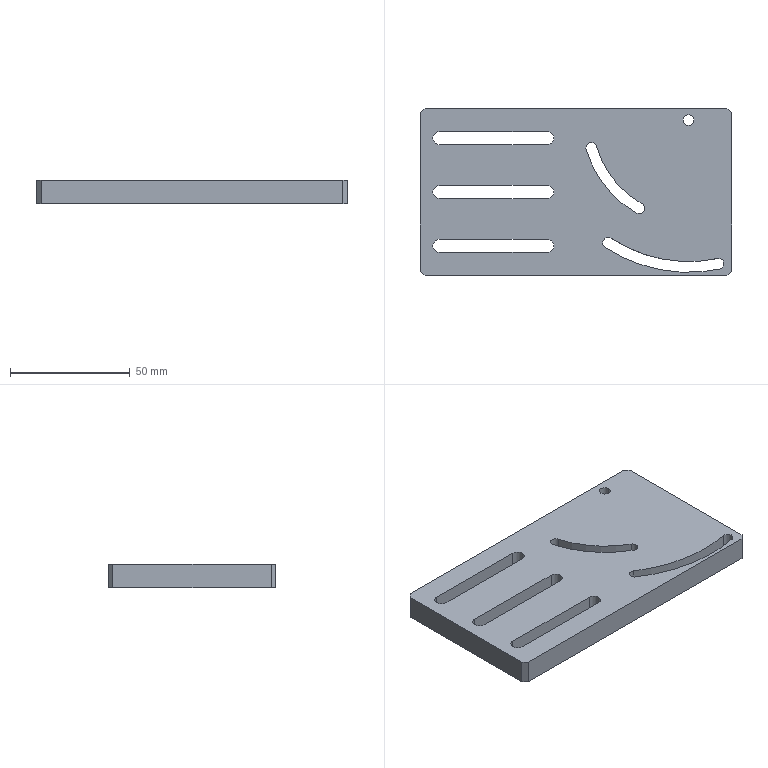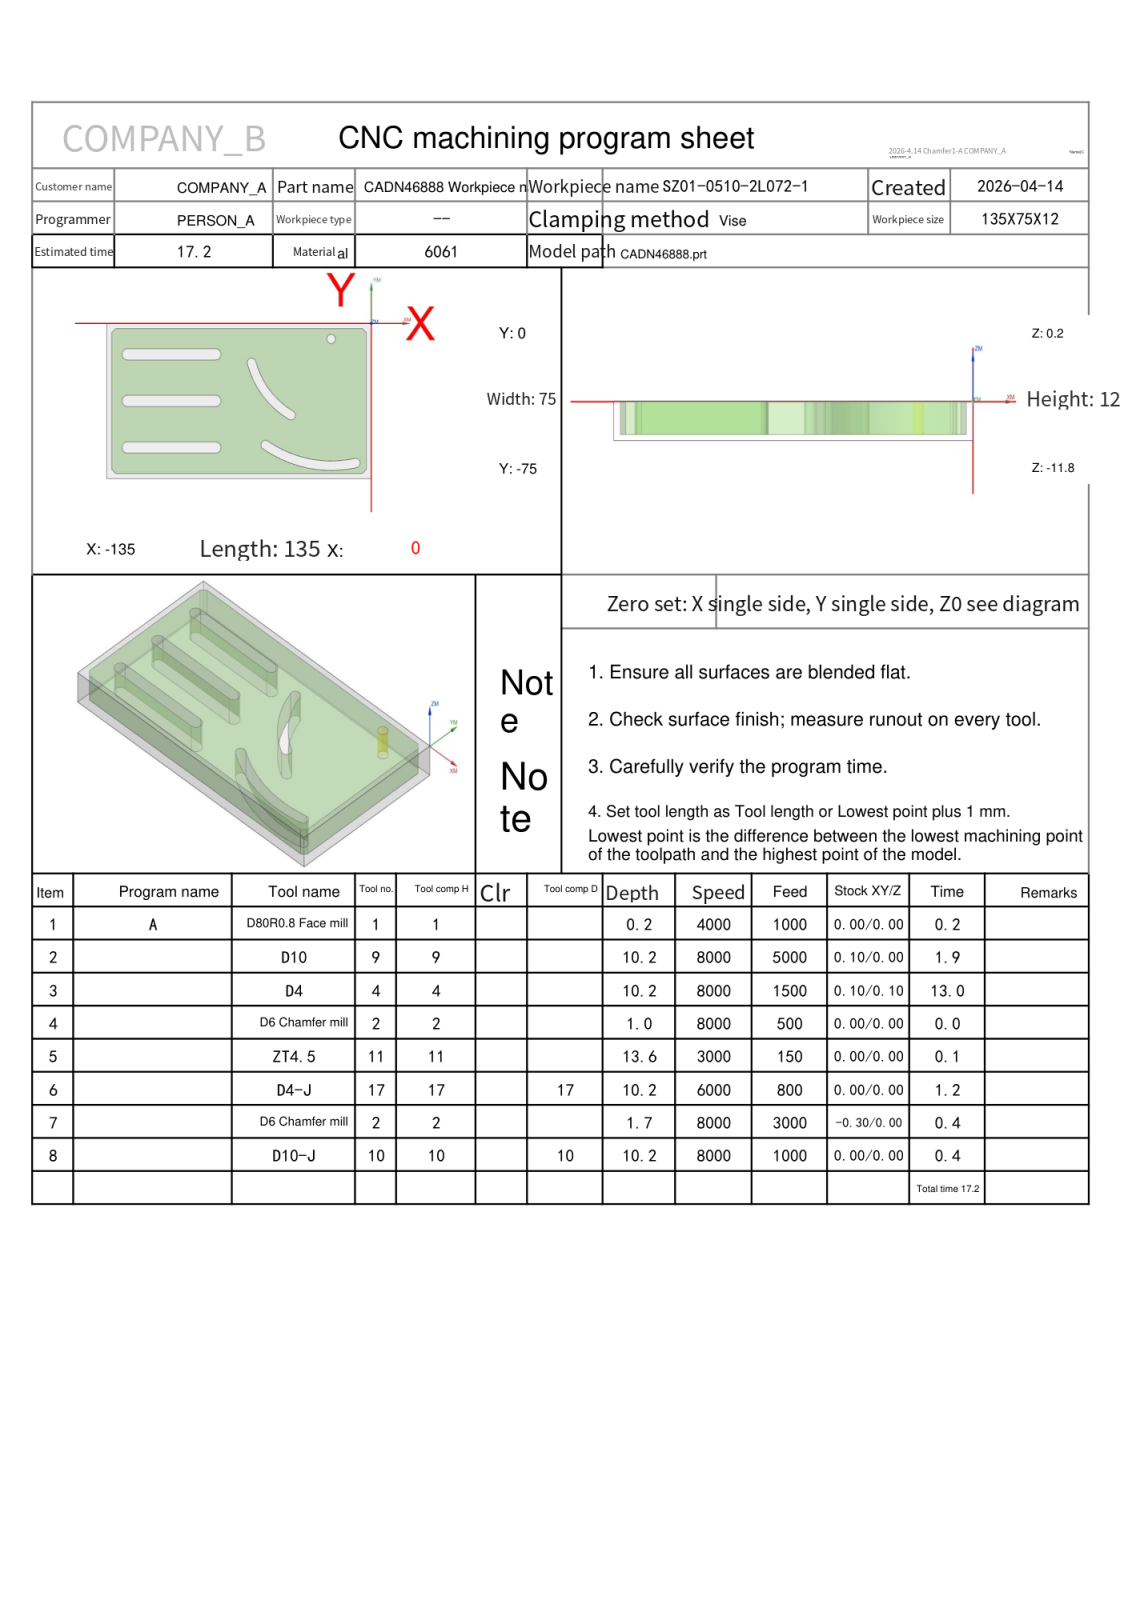NC program | NX | posted by the shop | part box 130 x 70 x 10 mm
Lines 448 to 1256 of 2533:
N5 T04 M06
(D4  D=4. R=0. H=04 ce=0.10 di=0.10)
G00 G90 G54 X-102. Y-60.65 M03 S8000
G43 H04 Z20.
M08
Z.5
G01 X-79.5 Z.442 F2500.
G03 X-78.85 Y-60. Z.439 I0.0 J.65
X-79.5 Y-59.35 Z.436 I-.65 J0.0
G01 X-124.5 Z.32
G03 X-125.15 Y-60. Z.317 I0.0 J-.65
X-124.89 Y-60.52 Z.315 I.65 J0.0
X-124.5 Y-60.65 Z.314 I.39 J.52
G01 X-79.5 Z.197
G03 X-78.85 Y-60. Z.195 I0.0 J.65
X-79.5 Y-59.35 Z.192 I-.65 J0.0
G01 X-124.5 Z.075
G03 X-125.15 Y-60. Z.073 I0.0 J-.65
X-124.89 Y-60.52 Z.071 I.65 J0.0
X-124.5 Y-60.65 Z.07 I.39 J.52
G01 X-79.5 Z-.047
G03 X-78.85 Y-60. Z-.049 I0.0 J.65
X-79.5 Y-59.35 Z-.052 I-.65 J0.0
G01 X-124.5 Z-.169
G03 X-125.15 Y-60. Z-.172 I0.0 J-.65
X-124.89 Y-60.52 Z-.173 I.65 J0.0
X-124.5 Y-60.65 Z-.174 I.39 J.52
G01 X-79.5 Z-.291
G03 X-78.85 Y-60. Z-.294 I0.0 J.65
X-79.5 Y-59.35 Z-.296 I-.65 J0.0
G01 X-124.5 Z-.413
G03 X-125.15 Y-60. Z-.416 I0.0 J-.65
X-124.89 Y-60.52 Z-.417 I.65 J0.0
X-124.5 Y-60.65 Z-.418 I.39 J.52
G01 X-79.5 Z-.535
G03 X-78.85 Y-60. Z-.538 I0.0 J.65
X-79.5 Y-59.35 Z-.54 I-.65 J0.0
G01 X-124.5 Z-.657
G03 X-125.15 Y-60. Z-.66 I0.0 J-.65
X-124.89 Y-60.52 Z-.661 I.65 J0.0
X-124.5 Y-60.65 Z-.663 I.39 J.52
G01 X-79.5 Z-.779
G03 X-78.85 Y-60. Z-.782 I0.0 J.65
X-79.5 Y-59.35 Z-.785 I-.65 J0.0
G01 X-124.5 Z-.901
G03 X-125.15 Y-60. Z-.904 I0.0 J-.65
X-124.89 Y-60.52 Z-.906 I.65 J0.0
X-124.5 Y-60.65 Z-.907 I.39 J.52
G01 X-79.5 Z-1.024
G03 X-78.85 Y-60. Z-1.026 I0.0 J.65
X-79.5 Y-59.35 Z-1.029 I-.65 J0.0
G01 X-124.5 Z-1.146
G03 X-125.15 Y-60. Z-1.148 I0.0 J-.65
X-124.89 Y-60.52 Z-1.15 I.65 J0.0
X-124.5 Y-60.65 Z-1.151 I.39 J.52
G01 X-79.5 Z-1.268
G03 X-78.85 Y-60. Z-1.27 I0.0 J.65
X-79.5 Y-59.35 Z-1.273 I-.65 J0.0
G01 X-124.5 Z-1.39
G03 X-125.15 Y-60. Z-1.392 I0.0 J-.65
X-124.89 Y-60.52 Z-1.394 I.65 J0.0
X-124.5 Y-60.65 Z-1.395 I.39 J.52
G01 X-79.5 Z-1.512
G03 X-78.85 Y-60. Z-1.515 I0.0 J.65
X-79.5 Y-59.35 Z-1.517 I-.65 J0.0
G01 X-124.5 Z-1.634
G03 X-125.15 Y-60. Z-1.637 I0.0 J-.65
X-124.89 Y-60.52 Z-1.638 I.65 J0.0
X-124.5 Y-60.65 Z-1.639 I.39 J.52
G01 X-79.5 Z-1.756
G03 X-78.85 Y-60. Z-1.759 I0.0 J.65
X-79.5 Y-59.35 Z-1.761 I-.65 J0.0
G01 X-124.5 Z-1.878
G03 X-125.15 Y-60. Z-1.881 I0.0 J-.65
X-124.89 Y-60.52 Z-1.882 I.65 J0.0
X-124.5 Y-60.65 Z-1.883 I.39 J.52
G01 X-79.5 Z-2.
G03 X-78.85 Y-60. Z-2.003 I0.0 J.65
X-79.5 Y-59.35 Z-2.006 I-.65 J0.0
G01 X-124.5 Z-2.122
G03 X-125.15 Y-60. Z-2.125 I0.0 J-.65
X-124.89 Y-60.52 Z-2.127 I.65 J0.0
X-124.5 Y-60.65 Z-2.128 I.39 J.52
G01 X-79.5 Z-2.244
G03 X-78.85 Y-60. Z-2.247 I0.0 J.65
X-79.5 Y-59.35 Z-2.25 I-.65 J0.0
G01 X-124.5 Z-2.367
G03 X-125.15 Y-60. Z-2.369 I0.0 J-.65
X-124.89 Y-60.52 Z-2.371 I.65 J0.0
X-124.5 Y-60.65 Z-2.372 I.39 J.52
G01 X-79.5 Z-2.489
G03 X-78.85 Y-60. Z-2.491 I0.0 J.65
X-79.5 Y-59.35 Z-2.494 I-.65 J0.0
G01 X-124.5 Z-2.611
G03 X-125.15 Y-60. Z-2.613 I0.0 J-.65
X-124.89 Y-60.52 Z-2.615 I.65 J0.0
X-124.5 Y-60.65 Z-2.616 I.39 J.52
G01 X-79.5 Z-2.733
G03 X-78.85 Y-60. Z-2.735 I0.0 J.65
X-79.5 Y-59.35 Z-2.738 I-.65 J0.0
G01 X-124.5 Z-2.855
G03 X-125.15 Y-60. Z-2.858 I0.0 J-.65
X-124.89 Y-60.52 Z-2.859 I.65 J0.0
X-124.5 Y-60.65 Z-2.86 I.39 J.52
G01 X-79.5 Z-2.977
G03 X-78.85 Y-60. Z-2.98 I0.0 J.65
X-79.5 Y-59.35 Z-2.982 I-.65 J0.0
G01 X-124.5 Z-3.099
G03 X-125.15 Y-60. Z-3.102 I0.0 J-.65
X-124.89 Y-60.52 Z-3.103 I.65 J0.0
X-124.5 Y-60.65 Z-3.104 I.39 J.52
G01 X-79.5 Z-3.221
G03 X-78.85 Y-60. Z-3.224 I0.0 J.65
X-79.5 Y-59.35 Z-3.226 I-.65 J0.0
G01 X-124.5 Z-3.343
G03 X-125.15 Y-60. Z-3.346 I0.0 J-.65
X-124.89 Y-60.52 Z-3.347 I.65 J0.0
X-124.5 Y-60.65 Z-3.349 I.39 J.52
G01 X-79.5 Z-3.465
G03 X-78.85 Y-60. Z-3.468 I0.0 J.65
X-79.5 Y-59.35 Z-3.471 I-.65 J0.0
G01 X-124.5 Z-3.587
G03 X-125.15 Y-60. Z-3.59 I0.0 J-.65
X-124.89 Y-60.52 Z-3.592 I.65 J0.0
X-124.5 Y-60.65 Z-3.593 I.39 J.52
G01 X-79.5 Z-3.71
G03 X-78.85 Y-60. Z-3.712 I0.0 J.65
X-79.5 Y-59.35 Z-3.715 I-.65 J0.0
G01 X-124.5 Z-3.832
G03 X-125.15 Y-60. Z-3.834 I0.0 J-.65
X-124.89 Y-60.52 Z-3.836 I.65 J0.0
X-124.5 Y-60.65 Z-3.837 I.39 J.52
G01 X-79.5 Z-3.954
G03 X-78.85 Y-60. Z-3.956 I0.0 J.65
X-79.5 Y-59.35 Z-3.959 I-.65 J0.0
G01 X-124.5 Z-4.076
G03 X-125.15 Y-60. Z-4.078 I0.0 J-.65
X-124.89 Y-60.52 Z-4.08 I.65 J0.0
X-124.5 Y-60.65 Z-4.081 I.39 J.52
G01 X-79.5 Z-4.198
G03 X-78.85 Y-60. Z-4.201 I0.0 J.65
X-79.5 Y-59.35 Z-4.203 I-.65 J0.0
G01 X-124.5 Z-4.32
G03 X-125.15 Y-60. Z-4.323 I0.0 J-.65
X-124.89 Y-60.52 Z-4.324 I.65 J0.0
X-124.5 Y-60.65 Z-4.325 I.39 J.52
G01 X-79.5 Z-4.442
G03 X-78.85 Y-60. Z-4.445 I0.0 J.65
X-79.5 Y-59.35 Z-4.447 I-.65 J0.0
G01 X-124.5 Z-4.564
G03 X-125.15 Y-60. Z-4.567 I0.0 J-.65
X-124.89 Y-60.52 Z-4.568 I.65 J0.0
X-124.5 Y-60.65 Z-4.57 I.39 J.52
G01 X-79.5 Z-4.686
G03 X-78.85 Y-60. Z-4.689 I0.0 J.65
X-79.5 Y-59.35 Z-4.692 I-.65 J0.0
G01 X-124.5 Z-4.808
G03 X-125.15 Y-60. Z-4.811 I0.0 J-.65
X-124.89 Y-60.52 Z-4.813 I.65 J0.0
X-124.5 Y-60.65 Z-4.814 I.39 J.52
G01 X-79.5 Z-4.93
G03 X-78.85 Y-60. Z-4.933 I0.0 J.65
X-79.5 Y-59.35 Z-4.936 I-.65 J0.0
G01 X-124.5 Z-5.053
G03 X-125.15 Y-60. Z-5.055 I0.0 J-.65
X-124.89 Y-60.52 Z-5.057 I.65 J0.0
X-124.5 Y-60.65 Z-5.058 I.39 J.52
G01 X-79.5 Z-5.175
G03 X-78.85 Y-60. Z-5.177 I0.0 J.65
X-79.5 Y-59.35 Z-5.18 I-.65 J0.0
G01 X-124.5 Z-5.297
G03 X-125.15 Y-60. Z-5.299 I0.0 J-.65
X-124.89 Y-60.52 Z-5.301 I.65 J0.0
X-124.5 Y-60.65 Z-5.302 I.39 J.52
G01 X-79.5 Z-5.419
G03 X-78.85 Y-60. Z-5.422 I0.0 J.65
X-79.5 Y-59.35 Z-5.424 I-.65 J0.0
G01 X-124.5 Z-5.541
G03 X-125.15 Y-60. Z-5.544 I0.0 J-.65
X-124.89 Y-60.52 Z-5.545 I.65 J0.0
X-124.5 Y-60.65 Z-5.546 I.39 J.52
G01 X-79.5 Z-5.663
G03 X-78.85 Y-60. Z-5.666 I0.0 J.65
X-79.5 Y-59.35 Z-5.668 I-.65 J0.0
G01 X-124.5 Z-5.785
G03 X-125.15 Y-60. Z-5.788 I0.0 J-.65
X-124.89 Y-60.52 Z-5.789 I.65 J0.0
X-124.5 Y-60.65 Z-5.79 I.39 J.52
G01 X-79.5 Z-5.907
G03 X-78.85 Y-60. Z-5.91 I0.0 J.65
X-79.5 Y-59.35 Z-5.913 I-.65 J0.0
G01 X-124.5 Z-6.029
G03 X-125.15 Y-60. Z-6.032 I0.0 J-.65
X-124.89 Y-60.52 Z-6.034 I.65 J0.0
X-124.5 Y-60.65 Z-6.035 I.39 J.52
G01 X-79.5 Z-6.151
G03 X-78.85 Y-60. Z-6.154 I0.0 J.65
X-79.5 Y-59.35 Z-6.157 I-.65 J0.0
G01 X-124.5 Z-6.274
G03 X-125.15 Y-60. Z-6.276 I0.0 J-.65
X-124.89 Y-60.52 Z-6.278 I.65 J0.0
X-124.5 Y-60.65 Z-6.279 I.39 J.52
G01 X-79.5 Z-6.396
G03 X-78.85 Y-60. Z-6.398 I0.0 J.65
X-79.5 Y-59.35 Z-6.401 I-.65 J0.0
G01 X-124.5 Z-6.518
G03 X-125.15 Y-60. Z-6.52 I0.0 J-.65
X-124.89 Y-60.52 Z-6.522 I.65 J0.0
X-124.5 Y-60.65 Z-6.523 I.39 J.52
G01 X-79.5 Z-6.64
G03 X-78.85 Y-60. Z-6.642 I0.0 J.65
X-79.5 Y-59.35 Z-6.645 I-.65 J0.0
G01 X-124.5 Z-6.762
G03 X-125.15 Y-60. Z-6.765 I0.0 J-.65
X-124.89 Y-60.52 Z-6.766 I.65 J0.0
X-124.5 Y-60.65 Z-6.767 I.39 J.52
G01 X-79.5 Z-6.884
G03 X-78.85 Y-60. Z-6.887 I0.0 J.65
X-79.5 Y-59.35 Z-6.889 I-.65 J0.0
G01 X-124.5 Z-7.006
G03 X-125.15 Y-60. Z-7.009 I0.0 J-.65
X-124.89 Y-60.52 Z-7.01 I.65 J0.0
X-124.5 Y-60.65 Z-7.011 I.39 J.52
G01 X-79.5 Z-7.128
G03 X-78.85 Y-60. Z-7.131 I0.0 J.65
X-79.5 Y-59.35 Z-7.133 I-.65 J0.0
G01 X-124.5 Z-7.25
G03 X-125.15 Y-60. Z-7.253 I0.0 J-.65
X-124.89 Y-60.52 Z-7.254 I.65 J0.0
X-124.5 Y-60.65 Z-7.256 I.39 J.52
G01 X-79.5 Z-7.372
G03 X-78.85 Y-60. Z-7.375 I0.0 J.65
X-79.5 Y-59.35 Z-7.378 I-.65 J0.0
G01 X-124.5 Z-7.494
G03 X-125.15 Y-60. Z-7.497 I0.0 J-.65
X-124.89 Y-60.52 Z-7.499 I.65 J0.0
X-124.5 Y-60.65 Z-7.5 I.39 J.52
G01 X-79.5 Z-7.617
G03 X-78.85 Y-60. Z-7.619 I0.0 J.65
X-79.5 Y-59.35 Z-7.622 I-.65 J0.0
G01 X-124.5 Z-7.739
G03 X-125.15 Y-60. Z-7.741 I0.0 J-.65
X-124.89 Y-60.52 Z-7.743 I.65 J0.0
X-124.5 Y-60.65 Z-7.744 I.39 J.52
G01 X-79.5 Z-7.861
G03 X-78.85 Y-60. Z-7.863 I0.0 J.65
X-79.5 Y-59.35 Z-7.866 I-.65 J0.0
G01 X-124.5 Z-7.983
G03 X-125.15 Y-60. Z-7.985 I0.0 J-.65
X-124.89 Y-60.52 Z-7.987 I.65 J0.0
X-124.5 Y-60.65 Z-7.988 I.39 J.52
G01 X-79.5 Z-8.105
G03 X-78.85 Y-60. Z-8.108 I0.0 J.65
X-79.5 Y-59.35 Z-8.11 I-.65 J0.0
G01 X-124.5 Z-8.227
G03 X-125.15 Y-60. Z-8.23 I0.0 J-.65
X-124.89 Y-60.52 Z-8.231 I.65 J0.0
X-124.5 Y-60.65 Z-8.232 I.39 J.52
G01 X-79.5 Z-8.349
G03 X-78.85 Y-60. Z-8.352 I0.0 J.65
X-79.5 Y-59.35 Z-8.354 I-.65 J0.0
G01 X-124.5 Z-8.471
G03 X-125.15 Y-60. Z-8.474 I0.0 J-.65
X-124.89 Y-60.52 Z-8.475 I.65 J0.0
X-124.5 Y-60.65 Z-8.476 I.39 J.52
G01 X-79.5 Z-8.593
G03 X-78.85 Y-60. Z-8.596 I0.0 J.65
X-79.5 Y-59.35 Z-8.599 I-.65 J0.0
G01 X-124.5 Z-8.715
G03 X-125.15 Y-60. Z-8.718 I0.0 J-.65
X-124.89 Y-60.52 Z-8.72 I.65 J0.0
X-124.5 Y-60.65 Z-8.721 I.39 J.52
G01 X-79.5 Z-8.837
G03 X-78.85 Y-60. Z-8.84 I0.0 J.65
X-79.5 Y-59.35 Z-8.843 I-.65 J0.0
G01 X-124.5 Z-8.96
G03 X-125.15 Y-60. Z-8.962 I0.0 J-.65
X-124.89 Y-60.52 Z-8.964 I.65 J0.0
X-124.5 Y-60.65 Z-8.965 I.39 J.52
G01 X-79.5 Z-9.082
G03 X-78.85 Y-60. Z-9.084 I0.0 J.65
X-79.5 Y-59.35 Z-9.087 I-.65 J0.0
G01 X-124.5 Z-9.204
G03 X-125.15 Y-60. Z-9.206 I0.0 J-.65
X-124.89 Y-60.52 Z-9.208 I.65 J0.0
X-124.5 Y-60.65 Z-9.209 I.39 J.52
G01 X-79.5 Z-9.326
G03 X-78.85 Y-60. Z-9.328 I0.0 J.65
X-79.5 Y-59.35 Z-9.331 I-.65 J0.0
G01 X-124.5 Z-9.448
G03 X-125.15 Y-60. Z-9.451 I0.0 J-.65
X-124.89 Y-60.52 Z-9.452 I.65 J0.0
X-124.5 Y-60.65 Z-9.453 I.39 J.52
G01 X-79.5 Z-9.57
G03 X-78.85 Y-60. Z-9.573 I0.0 J.65
X-79.5 Y-59.35 Z-9.575 I-.65 J0.0
G01 X-124.5 Z-9.692
G03 X-125.15 Y-60. Z-9.695 I0.0 J-.65
X-124.89 Y-60.52 Z-9.696 I.65 J0.0
X-124.5 Y-60.65 Z-9.697 I.39 J.52
G01 X-79.5 Z-9.814
G03 X-78.85 Y-60. Z-9.817 I0.0 J.65
X-79.5 Y-59.35 Z-9.82 I-.65 J0.0
G01 X-124.5 Z-9.936
G03 X-125.15 Y-60. Z-9.939 I0.0 J-.65
X-124.89 Y-60.52 Z-9.941 I.65 J0.0
X-124.5 Y-60.65 Z-9.942 I.39 J.52
G01 X-102. Z-10.
X-79.5
G03 X-78.85 Y-60. I0.0 J.65
X-79.5 Y-59.35 I-.65 J0.0
G01 X-124.5
G03 X-125.15 Y-60. I0.0 J-.65
X-124.5 Y-60.65 I.65 J0.0
G01 X-102.
X-101.5
Z-9.
G00 Z20.
X-102. Y-36.85
Z.5
G01 X-124.5 Z.442
G03 X-125.15 Y-37.5 Z.439 I0.0 J-.65
X-124.5 Y-38.15 Z.436 I.65 J0.0
G01 X-79.5 Z.32
G03 X-78.85 Y-37.5 Z.317 I0.0 J.65
X-79.5 Y-36.85 Z.314 I-.65 J0.0
G01 X-124.5 Z.197
G03 X-125.15 Y-37.5 Z.195 I0.0 J-.65
X-124.5 Y-38.15 Z.192 I.65 J0.0
G01 X-79.5 Z.075
G03 X-78.85 Y-37.5 Z.073 I0.0 J.65
X-79.5 Y-36.85 Z.07 I-.65 J0.0
G01 X-124.5 Z-.047
G03 X-125.15 Y-37.5 Z-.049 I0.0 J-.65
X-124.5 Y-38.15 Z-.052 I.65 J0.0
G01 X-79.5 Z-.169
G03 X-78.85 Y-37.5 Z-.172 I0.0 J.65
X-79.5 Y-36.85 Z-.174 I-.65 J0.0
G01 X-124.5 Z-.291
G03 X-125.15 Y-37.5 Z-.294 I0.0 J-.65
X-124.5 Y-38.15 Z-.296 I.65 J0.0
G01 X-79.5 Z-.413
G03 X-78.85 Y-37.5 Z-.416 I0.0 J.65
X-79.5 Y-36.85 Z-.418 I-.65 J0.0
G01 X-124.5 Z-.535
G03 X-125.15 Y-37.5 Z-.538 I0.0 J-.65
X-124.5 Y-38.15 Z-.54 I.65 J0.0
G01 X-79.5 Z-.657
G03 X-78.85 Y-37.5 Z-.66 I0.0 J.65
X-79.5 Y-36.85 Z-.663 I-.65 J0.0
G01 X-124.5 Z-.779
G03 X-125.15 Y-37.5 Z-.782 I0.0 J-.65
X-124.5 Y-38.15 Z-.785 I.65 J0.0
G01 X-79.5 Z-.901
G03 X-78.85 Y-37.5 Z-.904 I0.0 J.65
X-79.5 Y-36.85 Z-.907 I-.65 J0.0
G01 X-124.5 Z-1.024
G03 X-125.15 Y-37.5 Z-1.026 I0.0 J-.65
X-124.5 Y-38.15 Z-1.029 I.65 J0.0
G01 X-79.5 Z-1.146
G03 X-78.85 Y-37.5 Z-1.148 I0.0 J.65
X-79.5 Y-36.85 Z-1.151 I-.65 J0.0
G01 X-124.5 Z-1.268
G03 X-125.15 Y-37.5 Z-1.27 I0.0 J-.65
X-124.5 Y-38.15 Z-1.273 I.65 J0.0
G01 X-79.5 Z-1.39
G03 X-78.85 Y-37.5 Z-1.392 I0.0 J.65
X-79.5 Y-36.85 Z-1.395 I-.65 J0.0
G01 X-124.5 Z-1.512
G03 X-125.15 Y-37.5 Z-1.515 I0.0 J-.65
X-124.5 Y-38.15 Z-1.517 I.65 J0.0
G01 X-79.5 Z-1.634
G03 X-78.85 Y-37.5 Z-1.637 I0.0 J.65
X-79.5 Y-36.85 Z-1.639 I-.65 J0.0
G01 X-124.5 Z-1.756
G03 X-125.15 Y-37.5 Z-1.759 I0.0 J-.65
X-124.5 Y-38.15 Z-1.761 I.65 J0.0
G01 X-79.5 Z-1.878
G03 X-78.85 Y-37.5 Z-1.881 I0.0 J.65
X-79.5 Y-36.85 Z-1.883 I-.65 J0.0
G01 X-124.5 Z-2.
G03 X-125.15 Y-37.5 Z-2.003 I0.0 J-.65
X-124.5 Y-38.15 Z-2.006 I.65 J0.0
G01 X-79.5 Z-2.122
G03 X-78.85 Y-37.5 Z-2.125 I0.0 J.65
X-79.5 Y-36.85 Z-2.128 I-.65 J0.0
G01 X-124.5 Z-2.244
G03 X-125.15 Y-37.5 Z-2.247 I0.0 J-.65
X-124.5 Y-38.15 Z-2.25 I.65 J0.0
G01 X-79.5 Z-2.367
G03 X-78.85 Y-37.5 Z-2.369 I0.0 J.65
X-79.5 Y-36.85 Z-2.372 I-.65 J0.0
G01 X-124.5 Z-2.489
G03 X-125.15 Y-37.5 Z-2.491 I0.0 J-.65
X-124.5 Y-38.15 Z-2.494 I.65 J0.0
G01 X-79.5 Z-2.611
G03 X-78.85 Y-37.5 Z-2.613 I0.0 J.65
X-79.5 Y-36.85 Z-2.616 I-.65 J0.0
G01 X-124.5 Z-2.733
G03 X-125.15 Y-37.5 Z-2.735 I0.0 J-.65
X-124.5 Y-38.15 Z-2.738 I.65 J0.0
G01 X-79.5 Z-2.855
G03 X-78.85 Y-37.5 Z-2.858 I0.0 J.65
X-79.5 Y-36.85 Z-2.86 I-.65 J0.0
G01 X-124.5 Z-2.977
G03 X-125.15 Y-37.5 Z-2.98 I0.0 J-.65
X-124.5 Y-38.15 Z-2.982 I.65 J0.0
G01 X-79.5 Z-3.099
G03 X-78.85 Y-37.5 Z-3.102 I0.0 J.65
X-79.5 Y-36.85 Z-3.104 I-.65 J0.0
G01 X-124.5 Z-3.221
G03 X-125.15 Y-37.5 Z-3.224 I0.0 J-.65
X-124.5 Y-38.15 Z-3.226 I.65 J0.0
G01 X-79.5 Z-3.343
G03 X-78.85 Y-37.5 Z-3.346 I0.0 J.65
X-79.5 Y-36.85 Z-3.349 I-.65 J0.0
G01 X-124.5 Z-3.465
G03 X-125.15 Y-37.5 Z-3.468 I0.0 J-.65
X-124.5 Y-38.15 Z-3.471 I.65 J0.0
G01 X-79.5 Z-3.587
G03 X-78.85 Y-37.5 Z-3.59 I0.0 J.65
X-79.5 Y-36.85 Z-3.593 I-.65 J0.0
G01 X-124.5 Z-3.71
G03 X-125.15 Y-37.5 Z-3.712 I0.0 J-.65
X-124.5 Y-38.15 Z-3.715 I.65 J0.0
G01 X-79.5 Z-3.832
G03 X-78.85 Y-37.5 Z-3.834 I0.0 J.65
X-79.5 Y-36.85 Z-3.837 I-.65 J0.0
G01 X-124.5 Z-3.954
G03 X-125.15 Y-37.5 Z-3.956 I0.0 J-.65
X-124.5 Y-38.15 Z-3.959 I.65 J0.0
G01 X-79.5 Z-4.076
G03 X-78.85 Y-37.5 Z-4.078 I0.0 J.65
X-79.5 Y-36.85 Z-4.081 I-.65 J0.0
G01 X-124.5 Z-4.198
G03 X-125.15 Y-37.5 Z-4.201 I0.0 J-.65
X-124.5 Y-38.15 Z-4.203 I.65 J0.0
G01 X-79.5 Z-4.32
G03 X-78.85 Y-37.5 Z-4.323 I0.0 J.65
X-79.5 Y-36.85 Z-4.325 I-.65 J0.0
G01 X-124.5 Z-4.442
G03 X-125.15 Y-37.5 Z-4.445 I0.0 J-.65
X-124.5 Y-38.15 Z-4.447 I.65 J0.0
G01 X-79.5 Z-4.564
G03 X-78.85 Y-37.5 Z-4.567 I0.0 J.65
X-79.5 Y-36.85 Z-4.57 I-.65 J0.0
G01 X-124.5 Z-4.686
G03 X-125.15 Y-37.5 Z-4.689 I0.0 J-.65
X-124.5 Y-38.15 Z-4.692 I.65 J0.0
G01 X-79.5 Z-4.808
G03 X-78.85 Y-37.5 Z-4.811 I0.0 J.65
X-79.5 Y-36.85 Z-4.814 I-.65 J0.0
G01 X-124.5 Z-4.93
G03 X-125.15 Y-37.5 Z-4.933 I0.0 J-.65
X-124.5 Y-38.15 Z-4.936 I.65 J0.0
G01 X-79.5 Z-5.053
G03 X-78.85 Y-37.5 Z-5.055 I0.0 J.65
X-79.5 Y-36.85 Z-5.058 I-.65 J0.0
G01 X-124.5 Z-5.175
G03 X-125.15 Y-37.5 Z-5.177 I0.0 J-.65
X-124.5 Y-38.15 Z-5.18 I.65 J0.0
G01 X-79.5 Z-5.297
G03 X-78.85 Y-37.5 Z-5.299 I0.0 J.65
X-79.5 Y-36.85 Z-5.302 I-.65 J0.0
G01 X-124.5 Z-5.419
G03 X-125.15 Y-37.5 Z-5.422 I0.0 J-.65
X-124.5 Y-38.15 Z-5.424 I.65 J0.0
G01 X-79.5 Z-5.541
G03 X-78.85 Y-37.5 Z-5.544 I0.0 J.65
X-79.5 Y-36.85 Z-5.546 I-.65 J0.0
G01 X-124.5 Z-5.663
G03 X-125.15 Y-37.5 Z-5.666 I0.0 J-.65
X-124.5 Y-38.15 Z-5.668 I.65 J0.0
G01 X-79.5 Z-5.785
G03 X-78.85 Y-37.5 Z-5.788 I0.0 J.65
X-79.5 Y-36.85 Z-5.79 I-.65 J0.0
G01 X-124.5 Z-5.907
G03 X-125.15 Y-37.5 Z-5.91 I0.0 J-.65
X-124.5 Y-38.15 Z-5.913 I.65 J0.0
G01 X-79.5 Z-6.029
G03 X-78.85 Y-37.5 Z-6.032 I0.0 J.65
X-79.5 Y-36.85 Z-6.035 I-.65 J0.0
G01 X-124.5 Z-6.151
G03 X-125.15 Y-37.5 Z-6.154 I0.0 J-.65
X-124.5 Y-38.15 Z-6.157 I.65 J0.0
G01 X-79.5 Z-6.274
G03 X-78.85 Y-37.5 Z-6.276 I0.0 J.65
X-79.5 Y-36.85 Z-6.279 I-.65 J0.0
G01 X-124.5 Z-6.396
G03 X-125.15 Y-37.5 Z-6.398 I0.0 J-.65
X-124.5 Y-38.15 Z-6.401 I.65 J0.0
G01 X-79.5 Z-6.518
G03 X-78.85 Y-37.5 Z-6.52 I0.0 J.65
X-79.5 Y-36.85 Z-6.523 I-.65 J0.0
G01 X-124.5 Z-6.64
G03 X-125.15 Y-37.5 Z-6.642 I0.0 J-.65
X-124.5 Y-38.15 Z-6.645 I.65 J0.0
G01 X-79.5 Z-6.762
G03 X-78.85 Y-37.5 Z-6.765 I0.0 J.65
X-79.5 Y-36.85 Z-6.767 I-.65 J0.0
G01 X-124.5 Z-6.884
G03 X-125.15 Y-37.5 Z-6.887 I0.0 J-.65
X-124.5 Y-38.15 Z-6.889 I.65 J0.0
G01 X-79.5 Z-7.006
G03 X-78.85 Y-37.5 Z-7.009 I0.0 J.65
X-79.5 Y-36.85 Z-7.011 I-.65 J0.0
G01 X-124.5 Z-7.128
G03 X-125.15 Y-37.5 Z-7.131 I0.0 J-.65
X-124.5 Y-38.15 Z-7.133 I.65 J0.0
G01 X-79.5 Z-7.25
G03 X-78.85 Y-37.5 Z-7.253 I0.0 J.65
X-79.5 Y-36.85 Z-7.256 I-.65 J0.0
G01 X-124.5 Z-7.372
G03 X-125.15 Y-37.5 Z-7.375 I0.0 J-.65
X-124.5 Y-38.15 Z-7.378 I.65 J0.0
G01 X-79.5 Z-7.494
G03 X-78.85 Y-37.5 Z-7.497 I0.0 J.65
X-79.5 Y-36.85 Z-7.5 I-.65 J0.0
G01 X-124.5 Z-7.617
G03 X-125.15 Y-37.5 Z-7.619 I0.0 J-.65
X-124.5 Y-38.15 Z-7.622 I.65 J0.0
G01 X-79.5 Z-7.739
G03 X-78.85 Y-37.5 Z-7.741 I0.0 J.65
X-79.5 Y-36.85 Z-7.744 I-.65 J0.0
G01 X-124.5 Z-7.861
G03 X-125.15 Y-37.5 Z-7.863 I0.0 J-.65
X-124.5 Y-38.15 Z-7.866 I.65 J0.0
G01 X-79.5 Z-7.983
G03 X-78.85 Y-37.5 Z-7.985 I0.0 J.65
X-79.5 Y-36.85 Z-7.988 I-.65 J0.0
G01 X-124.5 Z-8.105
G03 X-125.15 Y-37.5 Z-8.108 I0.0 J-.65
X-124.5 Y-38.15 Z-8.11 I.65 J0.0
G01 X-79.5 Z-8.227
G03 X-78.85 Y-37.5 Z-8.23 I0.0 J.65
X-79.5 Y-36.85 Z-8.232 I-.65 J0.0
G01 X-124.5 Z-8.349
G03 X-125.15 Y-37.5 Z-8.352 I0.0 J-.65
X-124.5 Y-38.15 Z-8.354 I.65 J0.0
G01 X-79.5 Z-8.471
G03 X-78.85 Y-37.5 Z-8.474 I0.0 J.65
X-79.5 Y-36.85 Z-8.476 I-.65 J0.0
G01 X-124.5 Z-8.593
G03 X-125.15 Y-37.5 Z-8.596 I0.0 J-.65
X-124.5 Y-38.15 Z-8.599 I.65 J0.0
G01 X-79.5 Z-8.715
G03 X-78.85 Y-37.5 Z-8.718 I0.0 J.65
X-79.5 Y-36.85 Z-8.721 I-.65 J0.0
G01 X-124.5 Z-8.837
G03 X-125.15 Y-37.5 Z-8.84 I0.0 J-.65
X-124.5 Y-38.15 Z-8.843 I.65 J0.0
G01 X-79.5 Z-8.96
G03 X-78.85 Y-37.5 Z-8.962 I0.0 J.65
X-79.5 Y-36.85 Z-8.965 I-.65 J0.0
G01 X-124.5 Z-9.082
G03 X-125.15 Y-37.5 Z-9.084 I0.0 J-.65
X-124.5 Y-38.15 Z-9.087 I.65 J0.0
G01 X-79.5 Z-9.204
G03 X-78.85 Y-37.5 Z-9.206 I0.0 J.65
X-79.5 Y-36.85 Z-9.209 I-.65 J0.0
G01 X-124.5 Z-9.326
G03 X-125.15 Y-37.5 Z-9.328 I0.0 J-.65
X-124.5 Y-38.15 Z-9.331 I.65 J0.0
G01 X-79.5 Z-9.448
G03 X-78.85 Y-37.5 Z-9.451 I0.0 J.65
X-79.5 Y-36.85 Z-9.453 I-.65 J0.0
G01 X-124.5 Z-9.57
G03 X-125.15 Y-37.5 Z-9.573 I0.0 J-.65
X-124.5 Y-38.15 Z-9.575 I.65 J0.0
G01 X-79.5 Z-9.692
G03 X-78.85 Y-37.5 Z-9.695 I0.0 J.65
X-79.5 Y-36.85 Z-9.697 I-.65 J0.0
G01 X-124.5 Z-9.814
G03 X-125.15 Y-37.5 Z-9.817 I0.0 J-.65
X-124.5 Y-38.15 Z-9.82 I.65 J0.0
G01 X-79.5 Z-9.936
G03 X-78.85 Y-37.5 Z-9.939 I0.0 J.65
X-79.5 Y-36.85 Z-9.942 I-.65 J0.0
G01 X-102. Z-10.
X-124.5
G03 X-125.15 Y-37.5 I0.0 J-.65
X-124.5 Y-38.15 I.65 J0.0
G01 X-79.5
G03 X-78.85 Y-37.5 I0.0 J.65
X-79.5 Y-36.85 I-.65 J0.0
G01 X-102.
X-102.5
Z-9.
G00 Z20.
X-102. Y-14.35
Z.5
G01 X-124.5 Z.442
G03 X-125.15 Y-15. Z.439 I0.0 J-.65
X-124.5 Y-15.65 Z.436 I.65 J0.0
G01 X-79.5 Z.32
G03 X-78.85 Y-15. Z.317 I0.0 J.65
X-79.5 Y-14.35 Z.314 I-.65 J0.0
G01 X-124.5 Z.197
G03 X-125.15 Y-15. Z.195 I0.0 J-.65
X-124.5 Y-15.65 Z.192 I.65 J0.0
G01 X-79.5 Z.075
G03 X-78.85 Y-15. Z.073 I0.0 J.65
X-79.5 Y-14.35 Z.07 I-.65 J0.0
G01 X-124.5 Z-.047
G03 X-125.15 Y-15. Z-.049 I0.0 J-.65
X-124.5 Y-15.65 Z-.052 I.65 J0.0
G01 X-79.5 Z-.169
G03 X-78.85 Y-15. Z-.172 I0.0 J.65
X-79.5 Y-14.35 Z-.174 I-.65 J0.0
G01 X-124.5 Z-.291
G03 X-125.15 Y-15. Z-.294 I0.0 J-.65
X-124.5 Y-15.65 Z-.296 I.65 J0.0
G01 X-79.5 Z-.413
G03 X-78.85 Y-15. Z-.416 I0.0 J.65
X-79.5 Y-14.35 Z-.418 I-.65 J0.0
G01 X-124.5 Z-.535
G03 X-125.15 Y-15. Z-.538 I0.0 J-.65
X-124.5 Y-15.65 Z-.54 I.65 J0.0
G01 X-79.5 Z-.657
G03 X-78.85 Y-15. Z-.66 I0.0 J.65
X-79.5 Y-14.35 Z-.663 I-.65 J0.0
G01 X-124.5 Z-.779
G03 X-125.15 Y-15. Z-.782 I0.0 J-.65
X-124.5 Y-15.65 Z-.785 I.65 J0.0
G01 X-79.5 Z-.901
G03 X-78.85 Y-15. Z-.904 I0.0 J.65
X-79.5 Y-14.35 Z-.907 I-.65 J0.0
G01 X-124.5 Z-1.024
G03 X-125.15 Y-15. Z-1.026 I0.0 J-.65
X-124.5 Y-15.65 Z-1.029 I.65 J0.0
G01 X-79.5 Z-1.146
G03 X-78.85 Y-15. Z-1.148 I0.0 J.65
X-79.5 Y-14.35 Z-1.151 I-.65 J0.0
G01 X-124.5 Z-1.268
G03 X-125.15 Y-15. Z-1.27 I0.0 J-.65
X-124.5 Y-15.65 Z-1.273 I.65 J0.0
G01 X-79.5 Z-1.39
G03 X-78.85 Y-15. Z-1.392 I0.0 J.65
X-79.5 Y-14.35 Z-1.395 I-.65 J0.0
G01 X-124.5 Z-1.512
G03 X-125.15 Y-15. Z-1.515 I0.0 J-.65
X-124.5 Y-15.65 Z-1.517 I.65 J0.0
G01 X-79.5 Z-1.634
G03 X-78.85 Y-15. Z-1.637 I0.0 J.65
X-79.5 Y-14.35 Z-1.639 I-.65 J0.0
G01 X-124.5 Z-1.756
G03 X-125.15 Y-15. Z-1.759 I0.0 J-.65
X-124.5 Y-15.65 Z-1.761 I.65 J0.0
G01 X-79.5 Z-1.878
G03 X-78.85 Y-15. Z-1.881 I0.0 J.65
X-79.5 Y-14.35 Z-1.883 I-.65 J0.0
G01 X-124.5 Z-2.
G03 X-125.15 Y-15. Z-2.003 I0.0 J-.65
X-124.5 Y-15.65 Z-2.006 I.65 J0.0
G01 X-79.5 Z-2.122
G03 X-78.85 Y-15. Z-2.125 I0.0 J.65
X-79.5 Y-14.35 Z-2.128 I-.65 J0.0
G01 X-124.5 Z-2.244
G03 X-125.15 Y-15. Z-2.247 I0.0 J-.65
X-124.5 Y-15.65 Z-2.25 I.65 J0.0
G01 X-79.5 Z-2.367
G03 X-78.85 Y-15. Z-2.369 I0.0 J.65
X-79.5 Y-14.35 Z-2.372 I-.65 J0.0
G01 X-124.5 Z-2.489
G03 X-125.15 Y-15. Z-2.491 I0.0 J-.65
X-124.5 Y-15.65 Z-2.494 I.65 J0.0
G01 X-79.5 Z-2.611
G03 X-78.85 Y-15. Z-2.613 I0.0 J.65
X-79.5 Y-14.35 Z-2.616 I-.65 J0.0
G01 X-124.5 Z-2.733
G03 X-125.15 Y-15. Z-2.735 I0.0 J-.65
X-124.5 Y-15.65 Z-2.738 I.65 J0.0
G01 X-79.5 Z-2.855
G03 X-78.85 Y-15. Z-2.858 I0.0 J.65
X-79.5 Y-14.35 Z-2.86 I-.65 J0.0
G01 X-124.5 Z-2.977
G03 X-125.15 Y-15. Z-2.98 I0.0 J-.65
X-124.5 Y-15.65 Z-2.982 I.65 J0.0
G01 X-79.5 Z-3.099
G03 X-78.85 Y-15. Z-3.102 I0.0 J.65
X-79.5 Y-14.35 Z-3.104 I-.65 J0.0
G01 X-124.5 Z-3.221
G03 X-125.15 Y-15. Z-3.224 I0.0 J-.65
X-124.5 Y-15.65 Z-3.226 I.65 J0.0
G01 X-79.5 Z-3.343
G03 X-78.85 Y-15. Z-3.346 I0.0 J.65
X-79.5 Y-14.35 Z-3.349 I-.65 J0.0
G01 X-124.5 Z-3.465
G03 X-125.15 Y-15. Z-3.468 I0.0 J-.65
X-124.5 Y-15.65 Z-3.471 I.65 J0.0
G01 X-79.5 Z-3.587
G03 X-78.85 Y-15. Z-3.59 I0.0 J.65
X-79.5 Y-14.35 Z-3.593 I-.65 J0.0
G01 X-124.5 Z-3.71
G03 X-125.15 Y-15. Z-3.712 I0.0 J-.65
X-124.5 Y-15.65 Z-3.715 I.65 J0.0
G01 X-79.5 Z-3.832
G03 X-78.85 Y-15. Z-3.834 I0.0 J.65
X-79.5 Y-14.35 Z-3.837 I-.65 J0.0
G01 X-124.5 Z-3.954
G03 X-125.15 Y-15. Z-3.956 I0.0 J-.65
X-124.5 Y-15.65 Z-3.959 I.65 J0.0
G01 X-79.5 Z-4.076
G03 X-78.85 Y-15. Z-4.078 I0.0 J.65
X-79.5 Y-14.35 Z-4.081 I-.65 J0.0
G01 X-124.5 Z-4.198
G03 X-125.15 Y-15. Z-4.201 I0.0 J-.65
X-124.5 Y-15.65 Z-4.203 I.65 J0.0
G01 X-79.5 Z-4.32
G03 X-78.85 Y-15. Z-4.323 I0.0 J.65
X-79.5 Y-14.35 Z-4.325 I-.65 J0.0
G01 X-124.5 Z-4.442
G03 X-125.15 Y-15. Z-4.445 I0.0 J-.65
X-124.5 Y-15.65 Z-4.447 I.65 J0.0
G01 X-79.5 Z-4.564
G03 X-78.85 Y-15. Z-4.567 I0.0 J.65
X-79.5 Y-14.35 Z-4.57 I-.65 J0.0
G01 X-124.5 Z-4.686
G03 X-125.15 Y-15. Z-4.689 I0.0 J-.65
X-124.5 Y-15.65 Z-4.692 I.65 J0.0
G01 X-79.5 Z-4.808
G03 X-78.85 Y-15. Z-4.811 I0.0 J.65
X-79.5 Y-14.35 Z-4.814 I-.65 J0.0
G01 X-124.5 Z-4.93
G03 X-125.15 Y-15. Z-4.933 I0.0 J-.65
X-124.5 Y-15.65 Z-4.936 I.65 J0.0
G01 X-79.5 Z-5.053
G03 X-78.85 Y-15. Z-5.055 I0.0 J.65
X-79.5 Y-14.35 Z-5.058 I-.65 J0.0
G01 X-124.5 Z-5.175
G03 X-125.15 Y-15. Z-5.177 I0.0 J-.65
X-124.5 Y-15.65 Z-5.18 I.65 J0.0
G01 X-79.5 Z-5.297
G03 X-78.85 Y-15. Z-5.299 I0.0 J.65
X-79.5 Y-14.35 Z-5.302 I-.65 J0.0
G01 X-124.5 Z-5.419
G03 X-125.15 Y-15. Z-5.422 I0.0 J-.65
X-124.5 Y-15.65 Z-5.424 I.65 J0.0
G01 X-79.5 Z-5.541
G03 X-78.85 Y-15. Z-5.544 I0.0 J.65
X-79.5 Y-14.35 Z-5.546 I-.65 J0.0
G01 X-124.5 Z-5.663
G03 X-125.15 Y-15. Z-5.666 I0.0 J-.65
X-124.5 Y-15.65 Z-5.668 I.65 J0.0
G01 X-79.5 Z-5.785
G03 X-78.85 Y-15. Z-5.788 I0.0 J.65
X-79.5 Y-14.35 Z-5.79 I-.65 J0.0
G01 X-124.5 Z-5.907
G03 X-125.15 Y-15. Z-5.91 I0.0 J-.65
X-124.5 Y-15.65 Z-5.913 I.65 J0.0
G01 X-79.5 Z-6.029
G03 X-78.85 Y-15. Z-6.032 I0.0 J.65
X-79.5 Y-14.35 Z-6.035 I-.65 J0.0
G01 X-124.5 Z-6.151
G03 X-125.15 Y-15. Z-6.154 I0.0 J-.65
X-124.5 Y-15.65 Z-6.157 I.65 J0.0
G01 X-79.5 Z-6.274
G03 X-78.85 Y-15. Z-6.276 I0.0 J.65
X-79.5 Y-14.35 Z-6.279 I-.65 J0.0
G01 X-124.5 Z-6.396
G03 X-125.15 Y-15. Z-6.398 I0.0 J-.65
X-124.5 Y-15.65 Z-6.401 I.65 J0.0
G01 X-79.5 Z-6.518
G03 X-78.85 Y-15. Z-6.52 I0.0 J.65
X-79.5 Y-14.35 Z-6.523 I-.65 J0.0
G01 X-124.5 Z-6.64
G03 X-125.15 Y-15. Z-6.642 I0.0 J-.65
X-124.5 Y-15.65 Z-6.645 I.65 J0.0
G01 X-79.5 Z-6.762
G03 X-78.85 Y-15. Z-6.765 I0.0 J.65
X-79.5 Y-14.35 Z-6.767 I-.65 J0.0
G01 X-124.5 Z-6.884
G03 X-125.15 Y-15. Z-6.887 I0.0 J-.65
X-124.5 Y-15.65 Z-6.889 I.65 J0.0
G01 X-79.5 Z-7.006
G03 X-78.85 Y-15. Z-7.009 I0.0 J.65
X-79.5 Y-14.35 Z-7.011 I-.65 J0.0
G01 X-124.5 Z-7.128
G03 X-125.15 Y-15. Z-7.131 I0.0 J-.65
X-124.5 Y-15.65 Z-7.133 I.65 J0.0
G01 X-79.5 Z-7.25
G03 X-78.85 Y-15. Z-7.253 I0.0 J.65
X-79.5 Y-14.35 Z-7.256 I-.65 J0.0
G01 X-124.5 Z-7.372
G03 X-125.15 Y-15. Z-7.375 I0.0 J-.65
X-124.5 Y-15.65 Z-7.378 I.65 J0.0
G01 X-79.5 Z-7.494
G03 X-78.85 Y-15. Z-7.497 I0.0 J.65
X-79.5 Y-14.35 Z-7.5 I-.65 J0.0
G01 X-124.5 Z-7.617
G03 X-125.15 Y-15. Z-7.619 I0.0 J-.65
X-124.5 Y-15.65 Z-7.622 I.65 J0.0
G01 X-79.5 Z-7.739
G03 X-78.85 Y-15. Z-7.741 I0.0 J.65
X-79.5 Y-14.35 Z-7.744 I-.65 J0.0
G01 X-124.5 Z-7.861
G03 X-125.15 Y-15. Z-7.863 I0.0 J-.65
X-124.5 Y-15.65 Z-7.866 I.65 J0.0
G01 X-79.5 Z-7.983
G03 X-78.85 Y-15. Z-7.985 I0.0 J.65
X-79.5 Y-14.35 Z-7.988 I-.65 J0.0
G01 X-124.5 Z-8.105
G03 X-125.15 Y-15. Z-8.108 I0.0 J-.65
X-124.5 Y-15.65 Z-8.11 I.65 J0.0
G01 X-79.5 Z-8.227
G03 X-78.85 Y-15. Z-8.23 I0.0 J.65
X-79.5 Y-14.35 Z-8.232 I-.65 J0.0
G01 X-124.5 Z-8.349
G03 X-125.15 Y-15. Z-8.352 I0.0 J-.65